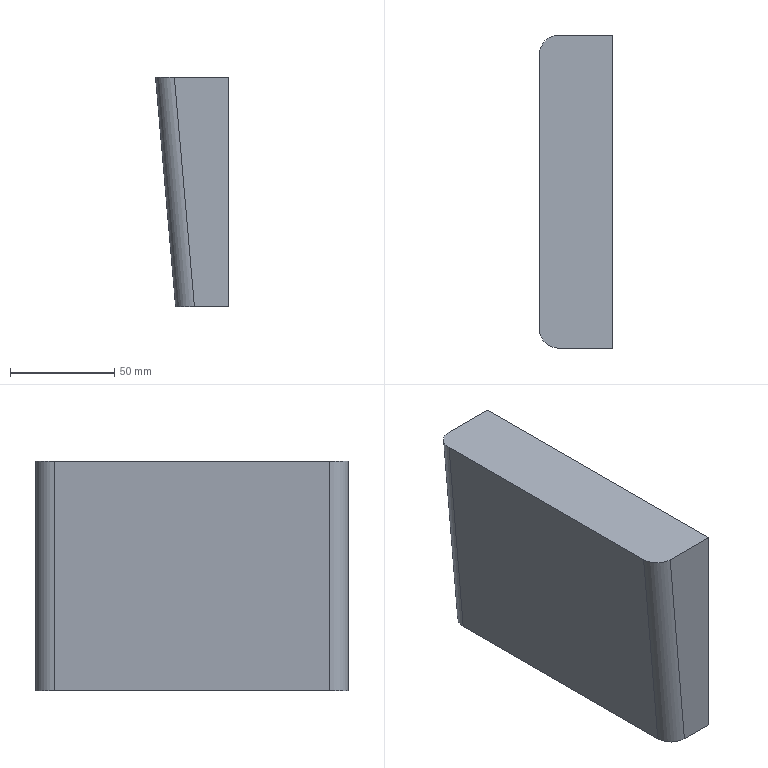Part | Creo | 1 solid | 8 faces | box 35 x 150 x 110 mm | volume 494266 mm3 | plane 6 | cylinder 2 | commonest cylinder face diameters 18 x2
STEP:
#1=CARTESIAN_POINT('',(0.,0.,0.));
#2=DIRECTION('',(0.,0.,1.));
#3=DIRECTION('',(1.,0.,0.));
#4=AXIS2_PLACEMENT_3D('',#1,#2,#3);
#5=CARTESIAN_POINT('',(-235.275,-230.589,-139.441));
#6=VERTEX_POINT('',#5);
#7=CARTESIAN_POINT('',(-235.275,-98.589,-139.441));
#8=VERTEX_POINT('',#7);
#9=CARTESIAN_POINT('',(-235.275,-230.589,-139.441));
#10=DIRECTION('',(0.,1.,0.));
#11=VECTOR('',#10,132.);
#12=LINE('',#9,#11);
#13=EDGE_CURVE('',#6,#8,#12,.T.);
#14=ORIENTED_EDGE('',*,*,#13,.T.);
#15=CARTESIAN_POINT('',(-244.899,-98.589,-29.441));
#16=VERTEX_POINT('',#15);
#17=CARTESIAN_POINT('',(-235.275,-98.589,-139.441));
#18=DIRECTION('',(-0.08716,0.,0.9962));
#19=VECTOR('',#18,110.42);
#20=LINE('',#17,#19);
#21=EDGE_CURVE('',#8,#16,#20,.T.);
#22=ORIENTED_EDGE('',*,*,#21,.T.);
#23=CARTESIAN_POINT('',(-244.899,-230.589,-29.441));
#24=VERTEX_POINT('',#23);
#25=CARTESIAN_POINT('',(-244.899,-230.589,-29.441));
#26=DIRECTION('',(0.,1.,0.));
#27=VECTOR('',#26,132.);
#28=LINE('',#25,#27);
#29=EDGE_CURVE('',#24,#16,#28,.T.);
#30=ORIENTED_EDGE('',*,*,#29,.F.);
#31=CARTESIAN_POINT('',(-244.899,-230.589,-29.441));
#32=DIRECTION('',(0.08716,0.,-0.9962));
#33=VECTOR('',#32,110.42);
#34=LINE('',#31,#33);
#35=EDGE_CURVE('',#24,#6,#34,.T.);
#36=ORIENTED_EDGE('',*,*,#35,.T.);
#37=EDGE_LOOP('',(#14,#22,#30,#36));
#38=FACE_OUTER_BOUND('',#37,.F.);
#39=CARTESIAN_POINT('',(-244.899,-119.589,-29.441));
#40=DIRECTION('',(0.9962,0.,0.08716));
#41=DIRECTION('',(0.08716,0.,-0.9962));
#42=AXIS2_PLACEMENT_3D('',#39,#40,#41);
#43=PLANE('',#42);
#44=ADVANCED_FACE('',(#38),#43,.F.);
#45=CARTESIAN_POINT('',(-209.899,-239.589,-139.441));
#46=VERTEX_POINT('',#45);
#47=CARTESIAN_POINT('',(-226.241,-239.589,-139.441));
#48=VERTEX_POINT('',#47);
#49=CARTESIAN_POINT('',(-209.899,-239.589,-139.441));
#50=DIRECTION('',(-1.,0.,0.));
#51=VECTOR('',#50,16.342);
#52=LINE('',#49,#51);
#53=EDGE_CURVE('',#46,#48,#52,.T.);
#54=ORIENTED_EDGE('',*,*,#53,.F.);
#55=CARTESIAN_POINT('',(-209.899,-89.589,-139.441));
#56=VERTEX_POINT('',#55);
#57=CARTESIAN_POINT('',(-209.899,-89.589,-139.441));
#58=DIRECTION('',(0.,-1.,0.));
#59=VECTOR('',#58,150.);
#60=LINE('',#57,#59);
#61=EDGE_CURVE('',#56,#46,#60,.T.);
#62=ORIENTED_EDGE('',*,*,#61,.F.);
#63=CARTESIAN_POINT('',(-226.241,-89.589,-139.441));
#64=VERTEX_POINT('',#63);
#65=CARTESIAN_POINT('',(-226.241,-89.589,-139.441));
#66=DIRECTION('',(1.,0.,0.));
#67=VECTOR('',#66,16.342);
#68=LINE('',#65,#67);
#69=EDGE_CURVE('',#64,#56,#68,.T.);
#70=ORIENTED_EDGE('',*,*,#69,.F.);
#71=CARTESIAN_POINT('',(-226.241,-89.589,-139.441));
#72=CARTESIAN_POINT('',(-226.992,-89.589,-139.441));
#73=CARTESIAN_POINT('',(-228.319,-89.766,-139.441));
#74=CARTESIAN_POINT('',(-230.552,-90.538,-139.441));
#75=CARTESIAN_POINT('',(-232.753,-92.095,-139.441));
#76=CARTESIAN_POINT('',(-234.318,-94.286,-139.441));
#77=CARTESIAN_POINT('',(-235.097,-96.513,-139.441));
#78=CARTESIAN_POINT('',(-235.275,-97.838,-139.441));
#79=CARTESIAN_POINT('',(-235.275,-98.589,-139.441));
#80=B_SPLINE_CURVE_WITH_KNOTS('',3,(#71,#72,#73,#74,#75,#76,#77,#78,#79),.UNSPECIFIED.,.F.,.F.,(4,1,1,1,1,1,4),(0.,0.125,0.25,0.5,0.75,0.875,1.),.UNSPECIFIED.);
#81=EDGE_CURVE('',#64,#8,#80,.T.);
#82=ORIENTED_EDGE('',*,*,#81,.T.);
#83=ORIENTED_EDGE('',*,*,#13,.F.);
#84=CARTESIAN_POINT('',(-235.275,-230.589,-139.441));
#85=CARTESIAN_POINT('',(-235.275,-231.341,-139.441));
#86=CARTESIAN_POINT('',(-235.097,-232.665,-139.441));
#87=CARTESIAN_POINT('',(-234.318,-234.892,-139.441));
#88=CARTESIAN_POINT('',(-232.753,-237.084,-139.441));
#89=CARTESIAN_POINT('',(-230.552,-238.64,-139.441));
#90=CARTESIAN_POINT('',(-228.319,-239.412,-139.441));
#91=CARTESIAN_POINT('',(-226.992,-239.589,-139.441));
#92=CARTESIAN_POINT('',(-226.241,-239.589,-139.441));
#93=B_SPLINE_CURVE_WITH_KNOTS('',3,(#84,#85,#86,#87,#88,#89,#90,#91,#92),.UNSPECIFIED.,.F.,.F.,(4,1,1,1,1,1,4),(0.,0.125,0.25,0.5,0.75,0.875,1.),.UNSPECIFIED.);
#94=EDGE_CURVE('',#6,#48,#93,.T.);
#95=ORIENTED_EDGE('',*,*,#94,.T.);
#96=EDGE_LOOP('',(#54,#62,#70,#82,#83,#95));
#97=FACE_OUTER_BOUND('',#96,.F.);
#98=CARTESIAN_POINT('',(-244.899,-239.589,-139.441));
#99=DIRECTION('',(0.,0.,1.));
#100=DIRECTION('',(1.,0.,0.));
#101=AXIS2_PLACEMENT_3D('',#98,#99,#100);
#102=PLANE('',#101);
#103=ADVANCED_FACE('',(#97),#102,.F.);
#104=CARTESIAN_POINT('',(-209.899,-239.589,-29.441));
#105=VERTEX_POINT('',#104);
#106=CARTESIAN_POINT('',(-235.865,-239.589,-29.441));
#107=VERTEX_POINT('',#106);
#108=CARTESIAN_POINT('',(-209.899,-239.589,-29.441));
#109=DIRECTION('',(-1.,0.,0.));
#110=VECTOR('',#109,25.966);
#111=LINE('',#108,#110);
#112=EDGE_CURVE('',#105,#107,#111,.T.);
#113=ORIENTED_EDGE('',*,*,#112,.F.);
#114=CARTESIAN_POINT('',(-209.899,-239.589,-29.441));
#115=DIRECTION('',(0.,0.,-1.));
#116=VECTOR('',#115,110.);
#117=LINE('',#114,#116);
#118=EDGE_CURVE('',#105,#46,#117,.T.);
#119=ORIENTED_EDGE('',*,*,#118,.T.);
#120=ORIENTED_EDGE('',*,*,#53,.T.);
#121=CARTESIAN_POINT('',(-235.865,-239.589,-29.441));
#122=DIRECTION('',(0.08716,0.,-0.9962));
#123=VECTOR('',#122,110.42);
#124=LINE('',#121,#123);
#125=EDGE_CURVE('',#107,#48,#124,.T.);
#126=ORIENTED_EDGE('',*,*,#125,.F.);
#127=EDGE_LOOP('',(#113,#119,#120,#126));
#128=FACE_OUTER_BOUND('',#127,.F.);
#129=CARTESIAN_POINT('',(-244.899,-239.589,-109.441));
#130=DIRECTION('',(0.,-1.,0.));
#131=DIRECTION('',(0.,0.,-1.));
#132=AXIS2_PLACEMENT_3D('',#129,#130,#131);
#133=PLANE('',#132);
#134=ADVANCED_FACE('',(#128),#133,.T.);
#135=ORIENTED_EDGE('',*,*,#29,.T.);
#136=CARTESIAN_POINT('',(-235.865,-89.589,-29.441));
#137=VERTEX_POINT('',#136);
#138=CARTESIAN_POINT('',(-244.899,-98.589,-29.441));
#139=CARTESIAN_POINT('',(-244.899,-97.838,-29.441));
#140=CARTESIAN_POINT('',(-244.721,-96.513,-29.441));
#141=CARTESIAN_POINT('',(-243.942,-94.286,-29.441));
#142=CARTESIAN_POINT('',(-242.376,-92.095,-29.441));
#143=CARTESIAN_POINT('',(-240.176,-90.538,-29.441));
#144=CARTESIAN_POINT('',(-237.942,-89.766,-29.441));
#145=CARTESIAN_POINT('',(-236.616,-89.589,-29.441));
#146=CARTESIAN_POINT('',(-235.865,-89.589,-29.441));
#147=B_SPLINE_CURVE_WITH_KNOTS('',3,(#138,#139,#140,#141,#142,#143,#144,#145,#146),.UNSPECIFIED.,.F.,.F.,(4,1,1,1,1,1,4),(0.,0.125,0.25,0.5,0.75,0.875,1.),.UNSPECIFIED.);
#148=EDGE_CURVE('',#16,#137,#147,.T.);
#149=ORIENTED_EDGE('',*,*,#148,.T.);
#150=CARTESIAN_POINT('',(-209.899,-89.589,-29.441));
#151=VERTEX_POINT('',#150);
#152=CARTESIAN_POINT('',(-235.865,-89.589,-29.441));
#153=DIRECTION('',(1.,0.,0.));
#154=VECTOR('',#153,25.966);
#155=LINE('',#152,#154);
#156=EDGE_CURVE('',#137,#151,#155,.T.);
#157=ORIENTED_EDGE('',*,*,#156,.T.);
#158=CARTESIAN_POINT('',(-209.899,-89.589,-29.441));
#159=DIRECTION('',(0.,-1.,0.));
#160=VECTOR('',#159,150.);
#161=LINE('',#158,#160);
#162=EDGE_CURVE('',#151,#105,#161,.T.);
#163=ORIENTED_EDGE('',*,*,#162,.T.);
#164=ORIENTED_EDGE('',*,*,#112,.T.);
#165=CARTESIAN_POINT('',(-235.865,-239.589,-29.441));
#166=CARTESIAN_POINT('',(-236.616,-239.589,-29.441));
#167=CARTESIAN_POINT('',(-237.942,-239.412,-29.441));
#168=CARTESIAN_POINT('',(-240.176,-238.64,-29.441));
#169=CARTESIAN_POINT('',(-242.376,-237.084,-29.441));
#170=CARTESIAN_POINT('',(-243.942,-234.892,-29.441));
#171=CARTESIAN_POINT('',(-244.721,-232.665,-29.441));
#172=CARTESIAN_POINT('',(-244.899,-231.341,-29.441));
#173=CARTESIAN_POINT('',(-244.899,-230.589,-29.441));
#174=B_SPLINE_CURVE_WITH_KNOTS('',3,(#165,#166,#167,#168,#169,#170,#171,#172,#173),.UNSPECIFIED.,.F.,.F.,(4,1,1,1,1,1,4),(0.,0.125,0.25,0.5,0.75,0.875,1.),.UNSPECIFIED.);
#175=EDGE_CURVE('',#107,#24,#174,.T.);
#176=ORIENTED_EDGE('',*,*,#175,.T.);
#177=EDGE_LOOP('',(#135,#149,#157,#163,#164,#176));
#178=FACE_OUTER_BOUND('',#177,.F.);
#179=CARTESIAN_POINT('',(-244.899,-239.589,-29.441));
#180=DIRECTION('',(0.,0.,1.));
#181=DIRECTION('',(1.,0.,0.));
#182=AXIS2_PLACEMENT_3D('',#179,#180,#181);
#183=PLANE('',#182);
#184=ADVANCED_FACE('',(#178),#183,.T.);
#185=ORIENTED_EDGE('',*,*,#81,.F.);
#186=CARTESIAN_POINT('',(-226.241,-89.589,-139.441));
#187=DIRECTION('',(-0.08716,0.,0.9962));
#188=VECTOR('',#187,110.42);
#189=LINE('',#186,#188);
#190=EDGE_CURVE('',#64,#137,#189,.T.);
#191=ORIENTED_EDGE('',*,*,#190,.T.);
#192=ORIENTED_EDGE('',*,*,#148,.F.);
#193=ORIENTED_EDGE('',*,*,#21,.F.);
#194=EDGE_LOOP('',(#185,#191,#192,#193));
#195=FACE_OUTER_BOUND('',#194,.F.);
#196=CARTESIAN_POINT('',(-228.722,-98.589,-111.088));
#197=DIRECTION('',(0.08716,0.,-0.9962));
#198=DIRECTION('',(-0.9962,0.,-0.08716));
#199=AXIS2_PLACEMENT_3D('',#196,#197,#198);
#200=CYLINDRICAL_SURFACE('',#199,9.);
#201=ADVANCED_FACE('',(#195),#200,.T.);
#202=ORIENTED_EDGE('',*,*,#69,.T.);
#203=CARTESIAN_POINT('',(-209.899,-89.589,-29.441));
#204=DIRECTION('',(0.,0.,-1.));
#205=VECTOR('',#204,110.);
#206=LINE('',#203,#205);
#207=EDGE_CURVE('',#151,#56,#206,.T.);
#208=ORIENTED_EDGE('',*,*,#207,.F.);
#209=ORIENTED_EDGE('',*,*,#156,.F.);
#210=ORIENTED_EDGE('',*,*,#190,.F.);
#211=EDGE_LOOP('',(#202,#208,#209,#210));
#212=FACE_OUTER_BOUND('',#211,.F.);
#213=CARTESIAN_POINT('',(-209.899,-89.589,-109.441));
#214=DIRECTION('',(0.,1.,0.));
#215=DIRECTION('',(0.,0.,1.));
#216=AXIS2_PLACEMENT_3D('',#213,#214,#215);
#217=PLANE('',#216);
#218=ADVANCED_FACE('',(#212),#217,.T.);
#219=ORIENTED_EDGE('',*,*,#162,.F.);
#220=ORIENTED_EDGE('',*,*,#207,.T.);
#221=ORIENTED_EDGE('',*,*,#61,.T.);
#222=ORIENTED_EDGE('',*,*,#118,.F.);
#223=EDGE_LOOP('',(#219,#220,#221,#222));
#224=FACE_OUTER_BOUND('',#223,.F.);
#225=CARTESIAN_POINT('',(-209.899,-239.589,-109.441));
#226=DIRECTION('',(1.,0.,0.));
#227=DIRECTION('',(0.,0.,-1.));
#228=AXIS2_PLACEMENT_3D('',#225,#226,#227);
#229=PLANE('',#228);
#230=ADVANCED_FACE('',(#224),#229,.T.);
#231=ORIENTED_EDGE('',*,*,#94,.F.);
#232=ORIENTED_EDGE('',*,*,#35,.F.);
#233=ORIENTED_EDGE('',*,*,#175,.F.);
#234=ORIENTED_EDGE('',*,*,#125,.T.);
#235=EDGE_LOOP('',(#231,#232,#233,#234));
#236=FACE_OUTER_BOUND('',#235,.F.);
#237=CARTESIAN_POINT('',(-235.933,-230.589,-28.657));
#238=DIRECTION('',(0.08716,0.,-0.9962));
#239=DIRECTION('',(-0.9962,0.,-0.08716));
#240=AXIS2_PLACEMENT_3D('',#237,#238,#239);
#241=CYLINDRICAL_SURFACE('',#240,9.);
#242=ADVANCED_FACE('',(#236),#241,.T.);
#243=CLOSED_SHELL('',(#44,#103,#134,#184,#201,#218,#230,#242));
#244=MANIFOLD_SOLID_BREP('',#243);
#245=(LENGTH_UNIT()NAMED_UNIT(*)SI_UNIT(.MILLI.,.METRE.));
#246=UNCERTAINTY_MEASURE_WITH_UNIT(LENGTH_MEASURE(0.01902),#245,'','');
#247=(NAMED_UNIT(*)PLANE_ANGLE_UNIT()SI_UNIT($,.RADIAN.));
#248=PLANE_ANGLE_MEASURE_WITH_UNIT(PLANE_ANGLE_MEASURE(0.01745),#247);
#249=(CONVERSION_BASED_UNIT('DEGREE',#248)NAMED_UNIT(*)PLANE_ANGLE_UNIT());
#250=(NAMED_UNIT(*)SI_UNIT($,.STERADIAN.)SOLID_ANGLE_UNIT());
#251=(GEOMETRIC_REPRESENTATION_CONTEXT(3)GLOBAL_UNCERTAINTY_ASSIGNED_CONTEXT((#246))GLOBAL_UNIT_ASSIGNED_CONTEXT((#245,#249,#250))REPRESENTATION_CONTEXT('',''));
#252=ADVANCED_BREP_SHAPE_REPRESENTATION('',(#4,#244),#251);